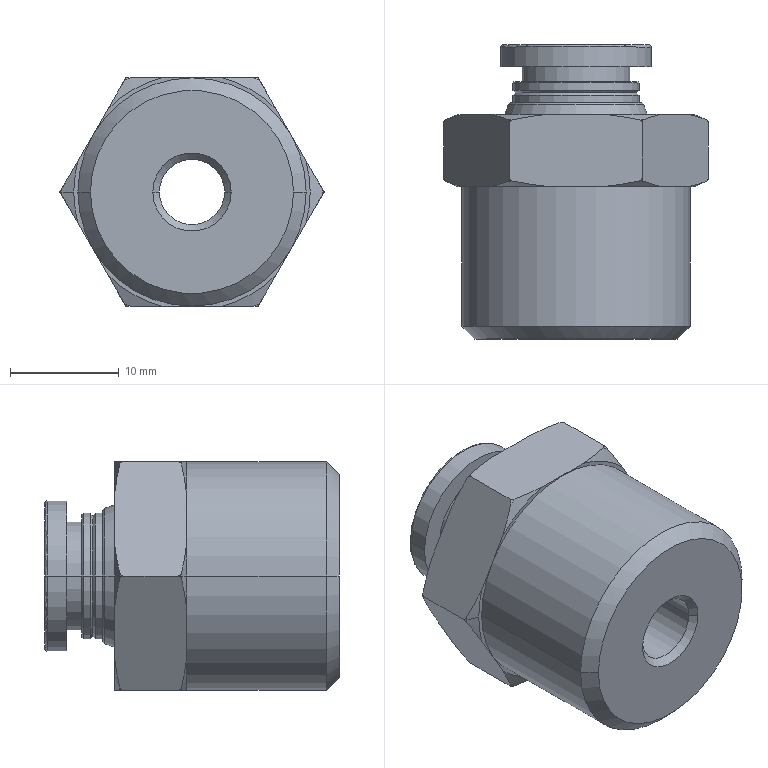Part | SolidWorks | features BaseBody 1 | 1 solid | 74 faces | box 24.249 x 27 x 21 mm | volume 6869 mm3 | cone 26 | torus 20 | cylinder 14 | plane 14 | commonest cylinder face diameters 11.6 x4 6 x2 8 x2 9.9 x2 13.8 x2 20.955 x2